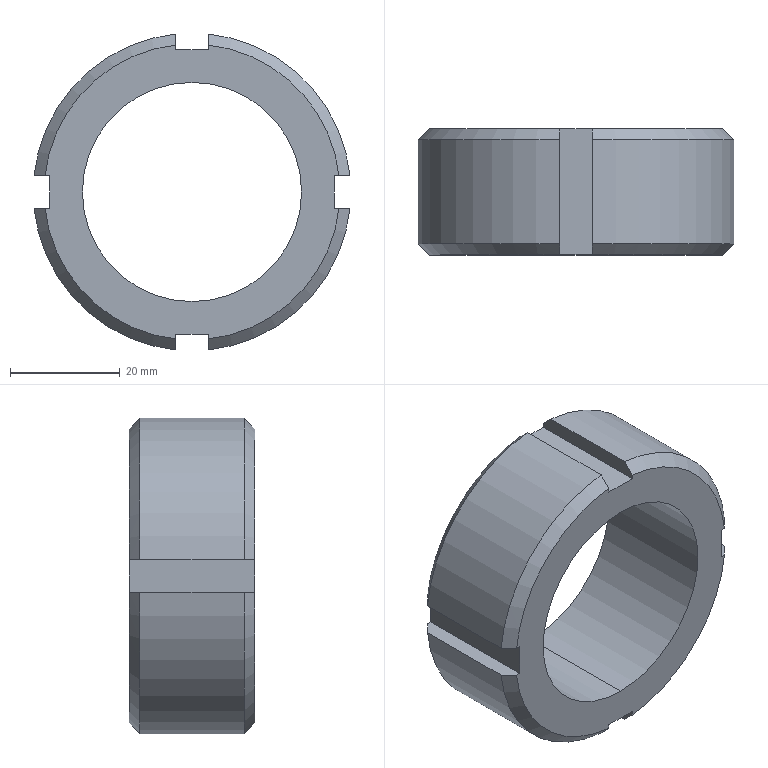Part | SolidWorks | features Chamfer 1, CirPattern 1, Extrusion 1, ICE 1 | 1 solid | 28 faces | box 57.689 x 23 x 57.689 mm | volume 29622 mm3 | plane 14 | cone 8 | cylinder 6 | commonest cylinder face diameters 58 x4 40 x2
STEP:
#1=CARTESIAN_POINT('',(0.,23.,-20.));
#2=VERTEX_POINT('',#1);
#3=CARTESIAN_POINT('',(0.,23.,20.));
#4=VERTEX_POINT('',#3);
#5=CARTESIAN_POINT('',(0.,23.,0.));
#6=DIRECTION('',(0.,1.,0.));
#7=DIRECTION('',(0.,0.,1.));
#8=AXIS2_PLACEMENT_3D('',#5,#6,#7);
#9=CIRCLE('',#8,20.);
#10=EDGE_CURVE('',#2,#4,#9,.T.);
#11=ORIENTED_EDGE('',*,*,#10,.T.);
#12=CARTESIAN_POINT('',(0.,0.,20.));
#13=VERTEX_POINT('',#12);
#14=CARTESIAN_POINT('',(0.,23.,20.));
#15=DIRECTION('',(0.,-1.,0.));
#16=VECTOR('',#15,1000.);
#17=LINE('',#14,#16);
#18=EDGE_CURVE('',#4,#13,#17,.T.);
#19=ORIENTED_EDGE('',*,*,#18,.T.);
#20=CARTESIAN_POINT('',(0.,0.,-20.));
#21=VERTEX_POINT('',#20);
#22=CARTESIAN_POINT('',(0.,0.,0.));
#23=DIRECTION('',(0.,1.,0.));
#24=DIRECTION('',(0.,0.,1.));
#25=AXIS2_PLACEMENT_3D('',#22,#23,#24);
#26=CIRCLE('',#25,20.);
#27=EDGE_CURVE('',#21,#13,#26,.T.);
#28=ORIENTED_EDGE('',*,*,#27,.F.);
#29=CARTESIAN_POINT('',(0.,23.,-20.));
#30=DIRECTION('',(0.,-1.,0.));
#31=VECTOR('',#30,1000.);
#32=LINE('',#29,#31);
#33=EDGE_CURVE('',#2,#21,#32,.T.);
#34=ORIENTED_EDGE('',*,*,#33,.F.);
#35=EDGE_LOOP('',(#11,#19,#28,#34));
#36=FACE_OUTER_BOUND('',#35,.T.);
#37=CARTESIAN_POINT('',(0.,23.,0.));
#38=DIRECTION('',(0.,-1.,0.));
#39=DIRECTION('',(0.,0.,-1.));
#40=AXIS2_PLACEMENT_3D('',#37,#38,#39);
#41=CYLINDRICAL_SURFACE('',#40,20.);
#42=ADVANCED_FACE('',(#36),#41,.F.);
#43=CARTESIAN_POINT('',(28.844,21.,3.));
#44=VERTEX_POINT('',#43);
#45=CARTESIAN_POINT('',(3.,21.,28.844));
#46=VERTEX_POINT('',#45);
#47=CARTESIAN_POINT('',(0.,21.,0.));
#48=DIRECTION('',(0.,-1.,0.));
#49=DIRECTION('',(0.,0.,1.));
#50=AXIS2_PLACEMENT_3D('',#47,#48,#49);
#51=CIRCLE('',#50,29.);
#52=EDGE_CURVE('',#44,#46,#51,.T.);
#53=ORIENTED_EDGE('',*,*,#52,.T.);
#54=CARTESIAN_POINT('',(3.,2.,28.844));
#55=VERTEX_POINT('',#54);
#56=CARTESIAN_POINT('',(3.,23.,28.844));
#57=DIRECTION('',(0.,-1.,0.));
#58=VECTOR('',#57,1000.);
#59=LINE('',#56,#58);
#60=EDGE_CURVE('',#46,#55,#59,.T.);
#61=ORIENTED_EDGE('',*,*,#60,.T.);
#62=CARTESIAN_POINT('',(28.844,2.,3.));
#63=VERTEX_POINT('',#62);
#64=CARTESIAN_POINT('',(0.,2.,0.));
#65=DIRECTION('',(0.,1.,0.));
#66=DIRECTION('',(0.,0.,1.));
#67=AXIS2_PLACEMENT_3D('',#64,#65,#66);
#68=CIRCLE('',#67,29.);
#69=EDGE_CURVE('',#55,#63,#68,.T.);
#70=ORIENTED_EDGE('',*,*,#69,.T.);
#71=CARTESIAN_POINT('',(28.844,23.,3.));
#72=DIRECTION('',(0.,1.,0.));
#73=VECTOR('',#72,1000.);
#74=LINE('',#71,#73);
#75=EDGE_CURVE('',#63,#44,#74,.T.);
#76=ORIENTED_EDGE('',*,*,#75,.T.);
#77=EDGE_LOOP('',(#53,#61,#70,#76));
#78=FACE_OUTER_BOUND('',#77,.T.);
#79=CARTESIAN_POINT('',(0.,23.,0.));
#80=DIRECTION('',(0.,-1.,0.));
#81=DIRECTION('',(0.,0.,-1.));
#82=AXIS2_PLACEMENT_3D('',#79,#80,#81);
#83=CYLINDRICAL_SURFACE('',#82,29.);
#84=ADVANCED_FACE('',(#78),#83,.T.);
#85=CARTESIAN_POINT('',(-28.844,2.,3.));
#86=VERTEX_POINT('',#85);
#87=CARTESIAN_POINT('',(-3.,2.,28.844));
#88=VERTEX_POINT('',#87);
#89=CARTESIAN_POINT('',(0.,2.,0.));
#90=DIRECTION('',(0.,1.,0.));
#91=DIRECTION('',(0.,0.,1.));
#92=AXIS2_PLACEMENT_3D('',#89,#90,#91);
#93=CIRCLE('',#92,29.);
#94=EDGE_CURVE('',#86,#88,#93,.T.);
#95=ORIENTED_EDGE('',*,*,#94,.T.);
#96=CARTESIAN_POINT('',(-3.,21.,28.844));
#97=VERTEX_POINT('',#96);
#98=CARTESIAN_POINT('',(-3.,23.,28.844));
#99=DIRECTION('',(0.,1.,0.));
#100=VECTOR('',#99,1000.);
#101=LINE('',#98,#100);
#102=EDGE_CURVE('',#88,#97,#101,.T.);
#103=ORIENTED_EDGE('',*,*,#102,.T.);
#104=CARTESIAN_POINT('',(-28.844,21.,3.));
#105=VERTEX_POINT('',#104);
#106=CARTESIAN_POINT('',(0.,21.,0.));
#107=DIRECTION('',(0.,-1.,0.));
#108=DIRECTION('',(0.,0.,1.));
#109=AXIS2_PLACEMENT_3D('',#106,#107,#108);
#110=CIRCLE('',#109,29.);
#111=EDGE_CURVE('',#97,#105,#110,.T.);
#112=ORIENTED_EDGE('',*,*,#111,.T.);
#113=CARTESIAN_POINT('',(-28.844,23.,3.));
#114=DIRECTION('',(0.,-1.,0.));
#115=VECTOR('',#114,1000.);
#116=LINE('',#113,#115);
#117=EDGE_CURVE('',#105,#86,#116,.T.);
#118=ORIENTED_EDGE('',*,*,#117,.T.);
#119=EDGE_LOOP('',(#95,#103,#112,#118));
#120=FACE_OUTER_BOUND('',#119,.T.);
#121=CARTESIAN_POINT('',(0.,23.,0.));
#122=DIRECTION('',(0.,-1.,0.));
#123=DIRECTION('',(0.,0.,-1.));
#124=AXIS2_PLACEMENT_3D('',#121,#122,#123);
#125=CYLINDRICAL_SURFACE('',#124,29.);
#126=ADVANCED_FACE('',(#120),#125,.T.);
#127=CARTESIAN_POINT('',(3.,0.,26.833));
#128=VERTEX_POINT('',#127);
#129=CARTESIAN_POINT('',(3.,0.,26.833));
#130=CARTESIAN_POINT('',(3.,0.1315,26.965));
#131=CARTESIAN_POINT('',(3.,0.263,27.097));
#132=CARTESIAN_POINT('',(3.,0.3946,27.23));
#133=CARTESIAN_POINT('',(3.,0.9296,27.768));
#134=CARTESIAN_POINT('',(3.,1.465,28.306));
#135=CARTESIAN_POINT('',(3.,2.,28.844));
#136=B_SPLINE_CURVE_WITH_KNOTS('',3,(#129,#130,#131,#132,#133,#134,#135),.UNSPECIFIED.,.F.,.F.,(4,3,4),(0.006406,0.006966,0.009243),.UNSPECIFIED.);
#137=EDGE_CURVE('',#128,#55,#136,.T.);
#138=ORIENTED_EDGE('',*,*,#137,.F.);
#139=CARTESIAN_POINT('',(26.833,0.,3.));
#140=VERTEX_POINT('',#139);
#141=CARTESIAN_POINT('',(0.,0.,0.));
#142=DIRECTION('',(0.,-1.,0.));
#143=DIRECTION('',(0.,0.,1.));
#144=AXIS2_PLACEMENT_3D('',#141,#142,#143);
#145=CIRCLE('',#144,27.);
#146=EDGE_CURVE('',#140,#128,#145,.T.);
#147=ORIENTED_EDGE('',*,*,#146,.F.);
#148=CARTESIAN_POINT('',(28.844,2.,3.));
#149=CARTESIAN_POINT('',(28.306,1.465,3.));
#150=CARTESIAN_POINT('',(27.768,0.9296,3.));
#151=CARTESIAN_POINT('',(27.23,0.3946,3.));
#152=CARTESIAN_POINT('',(27.097,0.263,3.));
#153=CARTESIAN_POINT('',(26.965,0.1315,3.));
#154=CARTESIAN_POINT('',(26.833,0.,3.));
#155=B_SPLINE_CURVE_WITH_KNOTS('',3,(#148,#149,#150,#151,#152,#153,#154),.UNSPECIFIED.,.F.,.F.,(4,3,4),(0.004689,0.006966,0.007525),.UNSPECIFIED.);
#156=EDGE_CURVE('',#63,#140,#155,.T.);
#157=ORIENTED_EDGE('',*,*,#156,.F.);
#158=ORIENTED_EDGE('',*,*,#69,.F.);
#159=EDGE_LOOP('',(#138,#147,#157,#158));
#160=FACE_OUTER_BOUND('',#159,.T.);
#161=CARTESIAN_POINT('',(0.,2.,0.));
#162=DIRECTION('',(0.,1.,0.));
#163=DIRECTION('',(0.,0.,1.));
#164=AXIS2_PLACEMENT_3D('',#161,#162,#163);
#165=CONICAL_SURFACE('',#164,29.,0.7854);
#166=ADVANCED_FACE('',(#160),#165,.T.);
#167=CARTESIAN_POINT('',(-3.,0.,26.833));
#168=VERTEX_POINT('',#167);
#169=CARTESIAN_POINT('',(-3.,2.,28.844));
#170=CARTESIAN_POINT('',(-3.,1.465,28.306));
#171=CARTESIAN_POINT('',(-3.,0.9296,27.768));
#172=CARTESIAN_POINT('',(-3.,0.3946,27.23));
#173=CARTESIAN_POINT('',(-3.,0.263,27.097));
#174=CARTESIAN_POINT('',(-3.,0.1315,26.965));
#175=CARTESIAN_POINT('',(-3.,0.,26.833));
#176=B_SPLINE_CURVE_WITH_KNOTS('',3,(#169,#170,#171,#172,#173,#174,#175),.UNSPECIFIED.,.F.,.F.,(4,3,4),(0.004689,0.006966,0.007525),.UNSPECIFIED.);
#177=EDGE_CURVE('',#88,#168,#176,.T.);
#178=ORIENTED_EDGE('',*,*,#177,.F.);
#179=ORIENTED_EDGE('',*,*,#94,.F.);
#180=CARTESIAN_POINT('',(-26.833,0.,3.));
#181=VERTEX_POINT('',#180);
#182=CARTESIAN_POINT('',(-26.833,0.,3.));
#183=CARTESIAN_POINT('',(-27.091,0.2565,3.));
#184=CARTESIAN_POINT('',(-27.349,0.513,3.));
#185=CARTESIAN_POINT('',(-27.607,0.7695,3.));
#186=CARTESIAN_POINT('',(-28.02,1.18,3.));
#187=CARTESIAN_POINT('',(-28.432,1.59,3.));
#188=CARTESIAN_POINT('',(-28.844,2.,3.));
#189=B_SPLINE_CURVE_WITH_KNOTS('',3,(#182,#183,#184,#185,#186,#187,#188),.UNSPECIFIED.,.F.,.F.,(4,3,4),(0.005874,0.006966,0.008711),.UNSPECIFIED.);
#190=EDGE_CURVE('',#181,#86,#189,.T.);
#191=ORIENTED_EDGE('',*,*,#190,.F.);
#192=CARTESIAN_POINT('',(0.,0.,0.));
#193=DIRECTION('',(0.,-1.,0.));
#194=DIRECTION('',(0.,0.,1.));
#195=AXIS2_PLACEMENT_3D('',#192,#193,#194);
#196=CIRCLE('',#195,27.);
#197=EDGE_CURVE('',#168,#181,#196,.T.);
#198=ORIENTED_EDGE('',*,*,#197,.F.);
#199=EDGE_LOOP('',(#178,#179,#191,#198));
#200=FACE_OUTER_BOUND('',#199,.T.);
#201=CARTESIAN_POINT('',(0.,2.,0.));
#202=DIRECTION('',(0.,1.,0.));
#203=DIRECTION('',(0.,0.,1.));
#204=AXIS2_PLACEMENT_3D('',#201,#202,#203);
#205=CONICAL_SURFACE('',#204,29.,0.7854);
#206=ADVANCED_FACE('',(#200),#205,.T.);
#207=CARTESIAN_POINT('',(3.,23.,26.833));
#208=VERTEX_POINT('',#207);
#209=CARTESIAN_POINT('',(3.,21.,28.844));
#210=CARTESIAN_POINT('',(3.,21.535,28.306));
#211=CARTESIAN_POINT('',(3.,22.07,27.768));
#212=CARTESIAN_POINT('',(3.,22.605,27.23));
#213=CARTESIAN_POINT('',(3.,22.737,27.097));
#214=CARTESIAN_POINT('',(3.,22.868,26.965));
#215=CARTESIAN_POINT('',(3.,23.,26.833));
#216=B_SPLINE_CURVE_WITH_KNOTS('',3,(#209,#210,#211,#212,#213,#214,#215),.UNSPECIFIED.,.F.,.F.,(4,3,4),(0.004689,0.006966,0.007525),.UNSPECIFIED.);
#217=EDGE_CURVE('',#46,#208,#216,.T.);
#218=ORIENTED_EDGE('',*,*,#217,.F.);
#219=ORIENTED_EDGE('',*,*,#52,.F.);
#220=CARTESIAN_POINT('',(26.833,23.,3.));
#221=VERTEX_POINT('',#220);
#222=CARTESIAN_POINT('',(26.833,23.,3.));
#223=CARTESIAN_POINT('',(26.965,22.868,3.));
#224=CARTESIAN_POINT('',(27.097,22.737,3.));
#225=CARTESIAN_POINT('',(27.23,22.605,3.));
#226=CARTESIAN_POINT('',(27.768,22.07,3.));
#227=CARTESIAN_POINT('',(28.306,21.535,3.));
#228=CARTESIAN_POINT('',(28.844,21.,3.));
#229=B_SPLINE_CURVE_WITH_KNOTS('',3,(#222,#223,#224,#225,#226,#227,#228),.UNSPECIFIED.,.F.,.F.,(4,3,4),(0.006406,0.006966,0.009243),.UNSPECIFIED.);
#230=EDGE_CURVE('',#221,#44,#229,.T.);
#231=ORIENTED_EDGE('',*,*,#230,.F.);
#232=CARTESIAN_POINT('',(0.,23.,0.));
#233=DIRECTION('',(0.,1.,0.));
#234=DIRECTION('',(0.,0.,1.));
#235=AXIS2_PLACEMENT_3D('',#232,#233,#234);
#236=CIRCLE('',#235,27.);
#237=EDGE_CURVE('',#208,#221,#236,.T.);
#238=ORIENTED_EDGE('',*,*,#237,.F.);
#239=EDGE_LOOP('',(#218,#219,#231,#238));
#240=FACE_OUTER_BOUND('',#239,.T.);
#241=CARTESIAN_POINT('',(0.,23.,0.));
#242=DIRECTION('',(0.,-1.,0.));
#243=DIRECTION('',(0.,0.,-1.));
#244=AXIS2_PLACEMENT_3D('',#241,#242,#243);
#245=CONICAL_SURFACE('',#244,27.,0.7854);
#246=ADVANCED_FACE('',(#240),#245,.T.);
#247=CARTESIAN_POINT('',(-3.,23.,26.833));
#248=VERTEX_POINT('',#247);
#249=CARTESIAN_POINT('',(-3.,23.,26.833));
#250=CARTESIAN_POINT('',(-3.,22.868,26.965));
#251=CARTESIAN_POINT('',(-3.,22.737,27.097));
#252=CARTESIAN_POINT('',(-3.,22.605,27.23));
#253=CARTESIAN_POINT('',(-3.,22.07,27.768));
#254=CARTESIAN_POINT('',(-3.,21.535,28.306));
#255=CARTESIAN_POINT('',(-3.,21.,28.844));
#256=B_SPLINE_CURVE_WITH_KNOTS('',3,(#249,#250,#251,#252,#253,#254,#255),.UNSPECIFIED.,.F.,.F.,(4,3,4),(0.006406,0.006966,0.009243),.UNSPECIFIED.);
#257=EDGE_CURVE('',#248,#97,#256,.T.);
#258=ORIENTED_EDGE('',*,*,#257,.F.);
#259=CARTESIAN_POINT('',(-26.833,23.,3.));
#260=VERTEX_POINT('',#259);
#261=CARTESIAN_POINT('',(0.,23.,0.));
#262=DIRECTION('',(0.,1.,0.));
#263=DIRECTION('',(0.,0.,1.));
#264=AXIS2_PLACEMENT_3D('',#261,#262,#263);
#265=CIRCLE('',#264,27.);
#266=EDGE_CURVE('',#260,#248,#265,.T.);
#267=ORIENTED_EDGE('',*,*,#266,.F.);
#268=CARTESIAN_POINT('',(-28.844,21.,3.));
#269=CARTESIAN_POINT('',(-28.724,21.119,3.));
#270=CARTESIAN_POINT('',(-28.604,21.239,3.));
#271=CARTESIAN_POINT('',(-28.484,21.358,3.));
#272=CARTESIAN_POINT('',(-27.934,21.906,3.));
#273=CARTESIAN_POINT('',(-27.383,22.453,3.));
#274=CARTESIAN_POINT('',(-26.833,23.,3.));
#275=B_SPLINE_CURVE_WITH_KNOTS('',3,(#268,#269,#270,#271,#272,#273,#274),.UNSPECIFIED.,.F.,.F.,(4,3,4),(0.006458,0.006966,0.009294),.UNSPECIFIED.);
#276=EDGE_CURVE('',#105,#260,#275,.T.);
#277=ORIENTED_EDGE('',*,*,#276,.F.);
#278=ORIENTED_EDGE('',*,*,#111,.F.);
#279=EDGE_LOOP('',(#258,#267,#277,#278));
#280=FACE_OUTER_BOUND('',#279,.T.);
#281=CARTESIAN_POINT('',(0.,23.,0.));
#282=DIRECTION('',(0.,-1.,0.));
#283=DIRECTION('',(0.,0.,-1.));
#284=AXIS2_PLACEMENT_3D('',#281,#282,#283);
#285=CONICAL_SURFACE('',#284,27.,0.7854);
#286=ADVANCED_FACE('',(#280),#285,.T.);
#287=CARTESIAN_POINT('',(3.,21.,-28.844));
#288=VERTEX_POINT('',#287);
#289=CARTESIAN_POINT('',(28.844,21.,-3.));
#290=VERTEX_POINT('',#289);
#291=CARTESIAN_POINT('',(0.,21.,0.));
#292=DIRECTION('',(0.,-1.,0.));
#293=DIRECTION('',(0.,0.,1.));
#294=AXIS2_PLACEMENT_3D('',#291,#292,#293);
#295=CIRCLE('',#294,29.);
#296=EDGE_CURVE('',#288,#290,#295,.T.);
#297=ORIENTED_EDGE('',*,*,#296,.T.);
#298=CARTESIAN_POINT('',(28.844,2.,-3.));
#299=VERTEX_POINT('',#298);
#300=CARTESIAN_POINT('',(28.844,23.,-3.));
#301=DIRECTION('',(0.,-1.,0.));
#302=VECTOR('',#301,1000.);
#303=LINE('',#300,#302);
#304=EDGE_CURVE('',#290,#299,#303,.T.);
#305=ORIENTED_EDGE('',*,*,#304,.T.);
#306=CARTESIAN_POINT('',(3.,2.,-28.844));
#307=VERTEX_POINT('',#306);
#308=CARTESIAN_POINT('',(0.,2.,0.));
#309=DIRECTION('',(0.,1.,0.));
#310=DIRECTION('',(0.,0.,1.));
#311=AXIS2_PLACEMENT_3D('',#308,#309,#310);
#312=CIRCLE('',#311,29.);
#313=EDGE_CURVE('',#299,#307,#312,.T.);
#314=ORIENTED_EDGE('',*,*,#313,.T.);
#315=CARTESIAN_POINT('',(3.,23.,-28.844));
#316=DIRECTION('',(0.,1.,0.));
#317=VECTOR('',#316,1000.);
#318=LINE('',#315,#317);
#319=EDGE_CURVE('',#307,#288,#318,.T.);
#320=ORIENTED_EDGE('',*,*,#319,.T.);
#321=EDGE_LOOP('',(#297,#305,#314,#320));
#322=FACE_OUTER_BOUND('',#321,.T.);
#323=CARTESIAN_POINT('',(0.,23.,0.));
#324=DIRECTION('',(0.,-1.,0.));
#325=DIRECTION('',(0.,0.,-1.));
#326=AXIS2_PLACEMENT_3D('',#323,#324,#325);
#327=CYLINDRICAL_SURFACE('',#326,29.);
#328=ADVANCED_FACE('',(#322),#327,.T.);
#329=CARTESIAN_POINT('',(26.833,0.,-3.));
#330=VERTEX_POINT('',#329);
#331=CARTESIAN_POINT('',(26.833,0.,-3.));
#332=CARTESIAN_POINT('',(26.965,0.1315,-3.));
#333=CARTESIAN_POINT('',(27.097,0.263,-3.));
#334=CARTESIAN_POINT('',(27.23,0.3946,-3.));
#335=CARTESIAN_POINT('',(27.768,0.9296,-3.));
#336=CARTESIAN_POINT('',(28.306,1.465,-3.));
#337=CARTESIAN_POINT('',(28.844,2.,-3.));
#338=B_SPLINE_CURVE_WITH_KNOTS('',3,(#331,#332,#333,#334,#335,#336,#337),.UNSPECIFIED.,.F.,.F.,(4,3,4),(0.006406,0.006966,0.009243),.UNSPECIFIED.);
#339=EDGE_CURVE('',#330,#299,#338,.T.);
#340=ORIENTED_EDGE('',*,*,#339,.F.);
#341=CARTESIAN_POINT('',(3.,0.,-26.833));
#342=VERTEX_POINT('',#341);
#343=CARTESIAN_POINT('',(0.,0.,0.));
#344=DIRECTION('',(0.,-1.,0.));
#345=DIRECTION('',(0.,0.,1.));
#346=AXIS2_PLACEMENT_3D('',#343,#344,#345);
#347=CIRCLE('',#346,27.);
#348=EDGE_CURVE('',#342,#330,#347,.T.);
#349=ORIENTED_EDGE('',*,*,#348,.F.);
#350=CARTESIAN_POINT('',(3.,2.,-28.844));
#351=CARTESIAN_POINT('',(3.,1.59,-28.432));
#352=CARTESIAN_POINT('',(3.,1.18,-28.02));
#353=CARTESIAN_POINT('',(3.,0.7695,-27.607));
#354=CARTESIAN_POINT('',(3.,0.513,-27.349));
#355=CARTESIAN_POINT('',(3.,0.2565,-27.091));
#356=CARTESIAN_POINT('',(3.,0.,-26.833));
#357=B_SPLINE_CURVE_WITH_KNOTS('',3,(#350,#351,#352,#353,#354,#355,#356),.UNSPECIFIED.,.F.,.F.,(4,3,4),(0.005221,0.006966,0.008057),.UNSPECIFIED.);
#358=EDGE_CURVE('',#307,#342,#357,.T.);
#359=ORIENTED_EDGE('',*,*,#358,.F.);
#360=ORIENTED_EDGE('',*,*,#313,.F.);
#361=EDGE_LOOP('',(#340,#349,#359,#360));
#362=FACE_OUTER_BOUND('',#361,.T.);
#363=CARTESIAN_POINT('',(0.,2.,0.));
#364=DIRECTION('',(0.,1.,0.));
#365=DIRECTION('',(0.,0.,1.));
#366=AXIS2_PLACEMENT_3D('',#363,#364,#365);
#367=CONICAL_SURFACE('',#366,29.,0.7854);
#368=ADVANCED_FACE('',(#362),#367,.T.);
#369=CARTESIAN_POINT('',(26.833,23.,-3.));
#370=VERTEX_POINT('',#369);
#371=CARTESIAN_POINT('',(28.844,21.,-3.));
#372=CARTESIAN_POINT('',(28.306,21.535,-3.));
#373=CARTESIAN_POINT('',(27.768,22.07,-3.));
#374=CARTESIAN_POINT('',(27.23,22.605,-3.));
#375=CARTESIAN_POINT('',(27.097,22.737,-3.));
#376=CARTESIAN_POINT('',(26.965,22.868,-3.));
#377=CARTESIAN_POINT('',(26.833,23.,-3.));
#378=B_SPLINE_CURVE_WITH_KNOTS('',3,(#371,#372,#373,#374,#375,#376,#377),.UNSPECIFIED.,.F.,.F.,(4,3,4),(0.004689,0.006966,0.007525),.UNSPECIFIED.);
#379=EDGE_CURVE('',#290,#370,#378,.T.);
#380=ORIENTED_EDGE('',*,*,#379,.F.);
#381=ORIENTED_EDGE('',*,*,#296,.F.);
#382=CARTESIAN_POINT('',(3.,23.,-26.833));
#383=VERTEX_POINT('',#382);
#384=CARTESIAN_POINT('',(3.,23.,-26.833));
#385=CARTESIAN_POINT('',(3.,22.453,-27.383));
#386=CARTESIAN_POINT('',(3.,21.906,-27.934));
#387=CARTESIAN_POINT('',(3.,21.358,-28.484));
#388=CARTESIAN_POINT('',(3.,21.239,-28.604));
#389=CARTESIAN_POINT('',(3.,21.119,-28.724));
#390=CARTESIAN_POINT('',(3.,21.,-28.844));
#391=B_SPLINE_CURVE_WITH_KNOTS('',3,(#384,#385,#386,#387,#388,#389,#390),.UNSPECIFIED.,.F.,.F.,(4,3,4),(0.004637,0.006966,0.007474),.UNSPECIFIED.);
#392=EDGE_CURVE('',#383,#288,#391,.T.);
#393=ORIENTED_EDGE('',*,*,#392,.F.);
#394=CARTESIAN_POINT('',(0.,23.,0.));
#395=DIRECTION('',(0.,1.,0.));
#396=DIRECTION('',(0.,0.,1.));
#397=AXIS2_PLACEMENT_3D('',#394,#395,#396);
#398=CIRCLE('',#397,27.);
#399=EDGE_CURVE('',#370,#383,#398,.T.);
#400=ORIENTED_EDGE('',*,*,#399,.F.);
#401=EDGE_LOOP('',(#380,#381,#393,#400));
#402=FACE_OUTER_BOUND('',#401,.T.);
#403=CARTESIAN_POINT('',(0.,23.,0.));
#404=DIRECTION('',(0.,-1.,0.));
#405=DIRECTION('',(0.,0.,-1.));
#406=AXIS2_PLACEMENT_3D('',#403,#404,#405);
#407=CONICAL_SURFACE('',#406,27.,0.7854);
#408=ADVANCED_FACE('',(#402),#407,.T.);
#409=CARTESIAN_POINT('',(3.,23.,26.));
#410=VERTEX_POINT('',#409);
#411=CARTESIAN_POINT('',(3.,23.,38.437));
#412=DIRECTION('',(0.,0.,-1.));
#413=VECTOR('',#412,1000.);
#414=LINE('',#411,#413);
#415=EDGE_CURVE('',#208,#410,#414,.T.);
#416=ORIENTED_EDGE('',*,*,#415,.F.);
#417=ORIENTED_EDGE('',*,*,#237,.T.);
#418=CARTESIAN_POINT('',(26.,23.,3.));
#419=VERTEX_POINT('',#418);
#420=CARTESIAN_POINT('',(38.437,23.,3.));
#421=DIRECTION('',(1.,0.,0.));
#422=VECTOR('',#421,1000.);
#423=LINE('',#420,#422);
#424=EDGE_CURVE('',#419,#221,#423,.T.);
#425=ORIENTED_EDGE('',*,*,#424,.F.);
#426=CARTESIAN_POINT('',(26.,23.,-3.));
#427=VERTEX_POINT('',#426);
#428=CARTESIAN_POINT('',(26.,23.,-3.));
#429=DIRECTION('',(0.,0.,1.));
#430=VECTOR('',#429,1000.);
#431=LINE('',#428,#430);
#432=EDGE_CURVE('',#427,#419,#431,.T.);
#433=ORIENTED_EDGE('',*,*,#432,.F.);
#434=CARTESIAN_POINT('',(38.437,23.,-3.));
#435=DIRECTION('',(-1.,0.,0.));
#436=VECTOR('',#435,1000.);
#437=LINE('',#434,#436);
#438=EDGE_CURVE('',#370,#427,#437,.T.);
#439=ORIENTED_EDGE('',*,*,#438,.F.);
#440=ORIENTED_EDGE('',*,*,#399,.T.);
#441=CARTESIAN_POINT('',(3.,23.,-26.));
#442=VERTEX_POINT('',#441);
#443=CARTESIAN_POINT('',(3.,23.,-38.437));
#444=DIRECTION('',(0.,0.,-1.));
#445=VECTOR('',#444,1000.);
#446=LINE('',#443,#445);
#447=EDGE_CURVE('',#442,#383,#446,.T.);
#448=ORIENTED_EDGE('',*,*,#447,.F.);
#449=CARTESIAN_POINT('',(-3.,23.,-26.));
#450=VERTEX_POINT('',#449);
#451=CARTESIAN_POINT('',(-3.,23.,-26.));
#452=DIRECTION('',(1.,0.,0.));
#453=VECTOR('',#452,1000.);
#454=LINE('',#451,#453);
#455=EDGE_CURVE('',#450,#442,#454,.T.);
#456=ORIENTED_EDGE('',*,*,#455,.F.);
#457=CARTESIAN_POINT('',(-3.,23.,-26.833));
#458=VERTEX_POINT('',#457);
#459=CARTESIAN_POINT('',(-3.,23.,-38.437));
#460=DIRECTION('',(0.,0.,1.));
#461=VECTOR('',#460,1000.);
#462=LINE('',#459,#461);
#463=EDGE_CURVE('',#458,#450,#462,.T.);
#464=ORIENTED_EDGE('',*,*,#463,.F.);
#465=CARTESIAN_POINT('',(-26.833,23.,-3.));
#466=VERTEX_POINT('',#465);
#467=CARTESIAN_POINT('',(0.,23.,0.));
#468=DIRECTION('',(0.,1.,0.));
#469=DIRECTION('',(0.,0.,1.));
#470=AXIS2_PLACEMENT_3D('',#467,#468,#469);
#471=CIRCLE('',#470,27.);
#472=EDGE_CURVE('',#458,#466,#471,.T.);
#473=ORIENTED_EDGE('',*,*,#472,.T.);
#474=CARTESIAN_POINT('',(-26.,23.,-3.));
#475=VERTEX_POINT('',#474);
#476=CARTESIAN_POINT('',(-38.437,23.,-3.));
#477=DIRECTION('',(-1.,0.,0.));
#478=VECTOR('',#477,1000.);
#479=LINE('',#476,#478);
#480=EDGE_CURVE('',#475,#466,#479,.T.);
#481=ORIENTED_EDGE('',*,*,#480,.F.);
#482=CARTESIAN_POINT('',(-26.,23.,3.));
#483=VERTEX_POINT('',#482);
#484=CARTESIAN_POINT('',(-26.,23.,3.));
#485=DIRECTION('',(0.,0.,-1.));
#486=VECTOR('',#485,1000.);
#487=LINE('',#484,#486);
#488=EDGE_CURVE('',#483,#475,#487,.T.);
#489=ORIENTED_EDGE('',*,*,#488,.F.);
#490=CARTESIAN_POINT('',(-38.437,23.,3.));
#491=DIRECTION('',(1.,0.,0.));
#492=VECTOR('',#491,1000.);
#493=LINE('',#490,#492);
#494=EDGE_CURVE('',#260,#483,#493,.T.);
#495=ORIENTED_EDGE('',*,*,#494,.F.);
#496=ORIENTED_EDGE('',*,*,#266,.T.);
#497=CARTESIAN_POINT('',(-3.,23.,26.));
#498=VERTEX_POINT('',#497);
#499=CARTESIAN_POINT('',(-3.,23.,38.437));
#500=DIRECTION('',(0.,0.,1.));
#501=VECTOR('',#500,1000.);
#502=LINE('',#499,#501);
#503=EDGE_CURVE('',#498,#248,#502,.T.);
#504=ORIENTED_EDGE('',*,*,#503,.F.);
#505=CARTESIAN_POINT('',(3.,23.,26.));
#506=DIRECTION('',(-1.,0.,0.));
#507=VECTOR('',#506,1000.);
#508=LINE('',#505,#507);
#509=EDGE_CURVE('',#410,#498,#508,.T.);
#510=ORIENTED_EDGE('',*,*,#509,.F.);
#511=EDGE_LOOP('',(#416,#417,#425,#433,#439,#440,#448,#456,#464,#473,#481,#489,#495,#496,#504,#510));
#512=FACE_OUTER_BOUND('',#511,.T.);
#513=ORIENTED_EDGE('',*,*,#10,.F.);
#514=CARTESIAN_POINT('',(0.,23.,0.));
#515=DIRECTION('',(0.,1.,0.));
#516=DIRECTION('',(0.,0.,1.));
#517=AXIS2_PLACEMENT_3D('',#514,#515,#516);
#518=CIRCLE('',#517,20.);
#519=EDGE_CURVE('',#4,#2,#518,.T.);
#520=ORIENTED_EDGE('',*,*,#519,.F.);
#521=EDGE_LOOP('',(#513,#520));
#522=FACE_BOUND('',#521,.T.);
#523=CARTESIAN_POINT('',(0.,23.,0.));
#524=DIRECTION('',(0.,1.,0.));
#525=DIRECTION('',(0.,0.,1.));
#526=AXIS2_PLACEMENT_3D('',#523,#524,#525);
#527=PLANE('',#526);
#528=ADVANCED_FACE('',(#512,#522),#527,.T.);
#529=ORIENTED_EDGE('',*,*,#146,.T.);
#530=CARTESIAN_POINT('',(3.,0.,26.));
#531=VERTEX_POINT('',#530);
#532=CARTESIAN_POINT('',(3.,0.,38.437));
#533=DIRECTION('',(0.,0.,-1.));
#534=VECTOR('',#533,1000.);
#535=LINE('',#532,#534);
#536=EDGE_CURVE('',#128,#531,#535,.T.);
#537=ORIENTED_EDGE('',*,*,#536,.T.);
#538=CARTESIAN_POINT('',(-3.,0.,26.));
#539=VERTEX_POINT('',#538);
#540=CARTESIAN_POINT('',(3.,0.,26.));
#541=DIRECTION('',(-1.,0.,0.));
#542=VECTOR('',#541,1000.);
#543=LINE('',#540,#542);
#544=EDGE_CURVE('',#531,#539,#543,.T.);
#545=ORIENTED_EDGE('',*,*,#544,.T.);
#546=CARTESIAN_POINT('',(-3.,0.,38.437));
#547=DIRECTION('',(0.,0.,1.));
#548=VECTOR('',#547,1000.);
#549=LINE('',#546,#548);
#550=EDGE_CURVE('',#539,#168,#549,.T.);
#551=ORIENTED_EDGE('',*,*,#550,.T.);
#552=ORIENTED_EDGE('',*,*,#197,.T.);
#553=CARTESIAN_POINT('',(-26.,0.,3.));
#554=VERTEX_POINT('',#553);
#555=CARTESIAN_POINT('',(-38.437,0.,3.));
#556=DIRECTION('',(1.,0.,0.));
#557=VECTOR('',#556,1000.);
#558=LINE('',#555,#557);
#559=EDGE_CURVE('',#181,#554,#558,.T.);
#560=ORIENTED_EDGE('',*,*,#559,.T.);
#561=CARTESIAN_POINT('',(-26.,0.,-3.));
#562=VERTEX_POINT('',#561);
#563=CARTESIAN_POINT('',(-26.,0.,3.));
#564=DIRECTION('',(0.,0.,-1.));
#565=VECTOR('',#564,1000.);
#566=LINE('',#563,#565);
#567=EDGE_CURVE('',#554,#562,#566,.T.);
#568=ORIENTED_EDGE('',*,*,#567,.T.);
#569=CARTESIAN_POINT('',(-26.833,0.,-3.));
#570=VERTEX_POINT('',#569);
#571=CARTESIAN_POINT('',(-38.437,0.,-3.));
#572=DIRECTION('',(-1.,0.,0.));
#573=VECTOR('',#572,1000.);
#574=LINE('',#571,#573);
#575=EDGE_CURVE('',#562,#570,#574,.T.);
#576=ORIENTED_EDGE('',*,*,#575,.T.);
#577=CARTESIAN_POINT('',(-3.,0.,-26.833));
#578=VERTEX_POINT('',#577);
#579=CARTESIAN_POINT('',(0.,0.,0.));
#580=DIRECTION('',(0.,-1.,0.));
#581=DIRECTION('',(0.,0.,1.));
#582=AXIS2_PLACEMENT_3D('',#579,#580,#581);
#583=CIRCLE('',#582,27.);
#584=EDGE_CURVE('',#570,#578,#583,.T.);
#585=ORIENTED_EDGE('',*,*,#584,.T.);
#586=CARTESIAN_POINT('',(-3.,0.,-26.));
#587=VERTEX_POINT('',#586);
#588=CARTESIAN_POINT('',(-3.,0.,-38.437));
#589=DIRECTION('',(0.,0.,1.));
#590=VECTOR('',#589,1000.);
#591=LINE('',#588,#590);
#592=EDGE_CURVE('',#578,#587,#591,.T.);
#593=ORIENTED_EDGE('',*,*,#592,.T.);
#594=CARTESIAN_POINT('',(3.,0.,-26.));
#595=VERTEX_POINT('',#594);
#596=CARTESIAN_POINT('',(-3.,0.,-26.));
#597=DIRECTION('',(1.,0.,0.));
#598=VECTOR('',#597,1000.);
#599=LINE('',#596,#598);
#600=EDGE_CURVE('',#587,#595,#599,.T.);
#601=ORIENTED_EDGE('',*,*,#600,.T.);
#602=CARTESIAN_POINT('',(3.,0.,-38.437));
#603=DIRECTION('',(0.,0.,-1.));
#604=VECTOR('',#603,1000.);
#605=LINE('',#602,#604);
#606=EDGE_CURVE('',#595,#342,#605,.T.);
#607=ORIENTED_EDGE('',*,*,#606,.T.);
#608=ORIENTED_EDGE('',*,*,#348,.T.);
#609=CARTESIAN_POINT('',(26.,0.,-3.));
#610=VERTEX_POINT('',#609);
#611=CARTESIAN_POINT('',(38.437,0.,-3.));
#612=DIRECTION('',(-1.,0.,0.));
#613=VECTOR('',#612,1000.);
#614=LINE('',#611,#613);
#615=EDGE_CURVE('',#330,#610,#614,.T.);
#616=ORIENTED_EDGE('',*,*,#615,.T.);
#617=CARTESIAN_POINT('',(26.,0.,3.));
#618=VERTEX_POINT('',#617);
#619=CARTESIAN_POINT('',(26.,0.,-3.));
#620=DIRECTION('',(0.,0.,1.));
#621=VECTOR('',#620,1000.);
#622=LINE('',#619,#621);
#623=EDGE_CURVE('',#610,#618,#622,.T.);
#624=ORIENTED_EDGE('',*,*,#623,.T.);
#625=CARTESIAN_POINT('',(38.437,0.,3.));
#626=DIRECTION('',(1.,0.,0.));
#627=VECTOR('',#626,1000.);
#628=LINE('',#625,#627);
#629=EDGE_CURVE('',#618,#140,#628,.T.);
#630=ORIENTED_EDGE('',*,*,#629,.T.);
#631=EDGE_LOOP('',(#529,#537,#545,#551,#552,#560,#568,#576,#585,#593,#601,#607,#608,#616,#624,#630));
#632=FACE_OUTER_BOUND('',#631,.T.);
#633=ORIENTED_EDGE('',*,*,#27,.T.);
#634=CARTESIAN_POINT('',(0.,0.,0.));
#635=DIRECTION('',(0.,1.,0.));
#636=DIRECTION('',(0.,0.,1.));
#637=AXIS2_PLACEMENT_3D('',#634,#635,#636);
#638=CIRCLE('',#637,20.);
#639=EDGE_CURVE('',#13,#21,#638,.T.);
#640=ORIENTED_EDGE('',*,*,#639,.T.);
#641=EDGE_LOOP('',(#633,#640));
#642=FACE_BOUND('',#641,.T.);
#643=CARTESIAN_POINT('',(0.,0.,0.));
#644=DIRECTION('',(0.,1.,0.));
#645=DIRECTION('',(0.,0.,1.));
#646=AXIS2_PLACEMENT_3D('',#643,#644,#645);
#647=PLANE('',#646);
#648=ADVANCED_FACE('',(#632,#642),#647,.F.);
#649=CARTESIAN_POINT('',(-3.,2.,-28.844));
#650=VERTEX_POINT('',#649);
#651=CARTESIAN_POINT('',(-28.844,2.,-3.));
#652=VERTEX_POINT('',#651);
#653=CARTESIAN_POINT('',(0.,2.,0.));
#654=DIRECTION('',(0.,1.,0.));
#655=DIRECTION('',(0.,0.,1.));
#656=AXIS2_PLACEMENT_3D('',#653,#654,#655);
#657=CIRCLE('',#656,29.);
#658=EDGE_CURVE('',#650,#652,#657,.T.);
#659=ORIENTED_EDGE('',*,*,#658,.T.);
#660=CARTESIAN_POINT('',(-28.844,21.,-3.));
#661=VERTEX_POINT('',#660);
#662=CARTESIAN_POINT('',(-28.844,23.,-3.));
#663=DIRECTION('',(0.,1.,0.));
#664=VECTOR('',#663,1000.);
#665=LINE('',#662,#664);
#666=EDGE_CURVE('',#652,#661,#665,.T.);
#667=ORIENTED_EDGE('',*,*,#666,.T.);
#668=CARTESIAN_POINT('',(-3.,21.,-28.844));
#669=VERTEX_POINT('',#668);
#670=CARTESIAN_POINT('',(0.,21.,0.));
#671=DIRECTION('',(0.,-1.,0.));
#672=DIRECTION('',(0.,0.,1.));
#673=AXIS2_PLACEMENT_3D('',#670,#671,#672);
#674=CIRCLE('',#673,29.);
#675=EDGE_CURVE('',#661,#669,#674,.T.);
#676=ORIENTED_EDGE('',*,*,#675,.T.);
#677=CARTESIAN_POINT('',(-3.,23.,-28.844));
#678=DIRECTION('',(0.,-1.,0.));
#679=VECTOR('',#678,1000.);
#680=LINE('',#677,#679);
#681=EDGE_CURVE('',#669,#650,#680,.T.);
#682=ORIENTED_EDGE('',*,*,#681,.T.);
#683=EDGE_LOOP('',(#659,#667,#676,#682));
#684=FACE_OUTER_BOUND('',#683,.T.);
#685=CARTESIAN_POINT('',(0.,23.,0.));
#686=DIRECTION('',(0.,-1.,0.));
#687=DIRECTION('',(0.,0.,-1.));
#688=AXIS2_PLACEMENT_3D('',#685,#686,#687);
#689=CYLINDRICAL_SURFACE('',#688,29.);
#690=ADVANCED_FACE('',(#684),#689,.T.);
#691=ORIENTED_EDGE('',*,*,#18,.F.);
#692=ORIENTED_EDGE('',*,*,#519,.T.);
#693=ORIENTED_EDGE('',*,*,#33,.T.);
#694=ORIENTED_EDGE('',*,*,#639,.F.);
#695=EDGE_LOOP('',(#691,#692,#693,#694));
#696=FACE_OUTER_BOUND('',#695,.T.);
#697=CARTESIAN_POINT('',(0.,23.,0.));
#698=DIRECTION('',(0.,-1.,0.));
#699=DIRECTION('',(0.,0.,-1.));
#700=AXIS2_PLACEMENT_3D('',#697,#698,#699);
#701=CYLINDRICAL_SURFACE('',#700,20.);
#702=ADVANCED_FACE('',(#696),#701,.F.);
#703=CARTESIAN_POINT('',(-28.844,2.,-3.));
#704=CARTESIAN_POINT('',(-28.432,1.59,-3.));
#705=CARTESIAN_POINT('',(-28.02,1.18,-3.));
#706=CARTESIAN_POINT('',(-27.607,0.7695,-3.));
#707=CARTESIAN_POINT('',(-27.349,0.513,-3.));
#708=CARTESIAN_POINT('',(-27.091,0.2565,-3.));
#709=CARTESIAN_POINT('',(-26.833,0.,-3.));
#710=B_SPLINE_CURVE_WITH_KNOTS('',3,(#703,#704,#705,#706,#707,#708,#709),.UNSPECIFIED.,.F.,.F.,(4,3,4),(0.005221,0.006966,0.008057),.UNSPECIFIED.);
#711=EDGE_CURVE('',#652,#570,#710,.T.);
#712=ORIENTED_EDGE('',*,*,#711,.F.);
#713=ORIENTED_EDGE('',*,*,#658,.F.);
#714=CARTESIAN_POINT('',(-3.,0.,-26.833));
#715=CARTESIAN_POINT('',(-3.,0.2565,-27.091));
#716=CARTESIAN_POINT('',(-3.,0.513,-27.349));
#717=CARTESIAN_POINT('',(-3.,0.7695,-27.607));
#718=CARTESIAN_POINT('',(-3.,1.18,-28.02));
#719=CARTESIAN_POINT('',(-3.,1.59,-28.432));
#720=CARTESIAN_POINT('',(-3.,2.,-28.844));
#721=B_SPLINE_CURVE_WITH_KNOTS('',3,(#714,#715,#716,#717,#718,#719,#720),.UNSPECIFIED.,.F.,.F.,(4,3,4),(0.005874,0.006966,0.008711),.UNSPECIFIED.);
#722=EDGE_CURVE('',#578,#650,#721,.T.);
#723=ORIENTED_EDGE('',*,*,#722,.F.);
#724=ORIENTED_EDGE('',*,*,#584,.F.);
#725=EDGE_LOOP('',(#712,#713,#723,#724));
#726=FACE_OUTER_BOUND('',#725,.T.);
#727=CARTESIAN_POINT('',(0.,2.,0.));
#728=DIRECTION('',(0.,1.,0.));
#729=DIRECTION('',(0.,0.,1.));
#730=AXIS2_PLACEMENT_3D('',#727,#728,#729);
#731=CONICAL_SURFACE('',#730,29.,0.7854);
#732=ADVANCED_FACE('',(#726),#731,.T.);
#733=CARTESIAN_POINT('',(-26.833,23.,-3.));
#734=CARTESIAN_POINT('',(-27.383,22.453,-3.));
#735=CARTESIAN_POINT('',(-27.934,21.906,-3.));
#736=CARTESIAN_POINT('',(-28.484,21.358,-3.));
#737=CARTESIAN_POINT('',(-28.604,21.239,-3.));
#738=CARTESIAN_POINT('',(-28.724,21.119,-3.));
#739=CARTESIAN_POINT('',(-28.844,21.,-3.));
#740=B_SPLINE_CURVE_WITH_KNOTS('',3,(#733,#734,#735,#736,#737,#738,#739),.UNSPECIFIED.,.F.,.F.,(4,3,4),(0.004637,0.006966,0.007474),.UNSPECIFIED.);
#741=EDGE_CURVE('',#466,#661,#740,.T.);
#742=ORIENTED_EDGE('',*,*,#741,.F.);
#743=ORIENTED_EDGE('',*,*,#472,.F.);
#744=CARTESIAN_POINT('',(-3.,21.,-28.844));
#745=CARTESIAN_POINT('',(-3.,21.119,-28.724));
#746=CARTESIAN_POINT('',(-3.,21.239,-28.604));
#747=CARTESIAN_POINT('',(-3.,21.358,-28.484));
#748=CARTESIAN_POINT('',(-3.,21.906,-27.934));
#749=CARTESIAN_POINT('',(-3.,22.453,-27.383));
#750=CARTESIAN_POINT('',(-3.,23.,-26.833));
#751=B_SPLINE_CURVE_WITH_KNOTS('',3,(#744,#745,#746,#747,#748,#749,#750),.UNSPECIFIED.,.F.,.F.,(4,3,4),(0.006458,0.006966,0.009294),.UNSPECIFIED.);
#752=EDGE_CURVE('',#669,#458,#751,.T.);
#753=ORIENTED_EDGE('',*,*,#752,.F.);
#754=ORIENTED_EDGE('',*,*,#675,.F.);
#755=EDGE_LOOP('',(#742,#743,#753,#754));
#756=FACE_OUTER_BOUND('',#755,.T.);
#757=CARTESIAN_POINT('',(0.,23.,0.));
#758=DIRECTION('',(0.,-1.,0.));
#759=DIRECTION('',(0.,0.,-1.));
#760=AXIS2_PLACEMENT_3D('',#757,#758,#759);
#761=CONICAL_SURFACE('',#760,27.,0.7854);
#762=ADVANCED_FACE('',(#756),#761,.T.);
#763=ORIENTED_EDGE('',*,*,#722,.T.);
#764=ORIENTED_EDGE('',*,*,#681,.F.);
#765=ORIENTED_EDGE('',*,*,#752,.T.);
#766=ORIENTED_EDGE('',*,*,#463,.T.);
#767=CARTESIAN_POINT('',(-3.,0.,-26.));
#768=DIRECTION('',(0.,1.,0.));
#769=VECTOR('',#768,1000.);
#770=LINE('',#767,#769);
#771=EDGE_CURVE('',#587,#450,#770,.T.);
#772=ORIENTED_EDGE('',*,*,#771,.F.);
#773=ORIENTED_EDGE('',*,*,#592,.F.);
#774=EDGE_LOOP('',(#763,#764,#765,#766,#772,#773));
#775=FACE_OUTER_BOUND('',#774,.T.);
#776=CARTESIAN_POINT('',(-3.,0.,-38.437));
#777=DIRECTION('',(-1.,0.,0.));
#778=DIRECTION('',(0.,0.,1.));
#779=AXIS2_PLACEMENT_3D('',#776,#777,#778);
#780=PLANE('',#779);
#781=ADVANCED_FACE('',(#775),#780,.F.);
#782=ORIENTED_EDGE('',*,*,#358,.T.);
#783=ORIENTED_EDGE('',*,*,#606,.F.);
#784=CARTESIAN_POINT('',(3.,0.,-26.));
#785=DIRECTION('',(0.,1.,0.));
#786=VECTOR('',#785,1000.);
#787=LINE('',#784,#786);
#788=EDGE_CURVE('',#595,#442,#787,.T.);
#789=ORIENTED_EDGE('',*,*,#788,.T.);
#790=ORIENTED_EDGE('',*,*,#447,.T.);
#791=ORIENTED_EDGE('',*,*,#392,.T.);
#792=ORIENTED_EDGE('',*,*,#319,.F.);
#793=EDGE_LOOP('',(#782,#783,#789,#790,#791,#792));
#794=FACE_OUTER_BOUND('',#793,.T.);
#795=CARTESIAN_POINT('',(3.,0.,-38.437));
#796=DIRECTION('',(1.,0.,0.));
#797=DIRECTION('',(0.,0.,-1.));
#798=AXIS2_PLACEMENT_3D('',#795,#796,#797);
#799=PLANE('',#798);
#800=ADVANCED_FACE('',(#794),#799,.F.);
#801=ORIENTED_EDGE('',*,*,#455,.T.);
#802=ORIENTED_EDGE('',*,*,#788,.F.);
#803=ORIENTED_EDGE('',*,*,#600,.F.);
#804=ORIENTED_EDGE('',*,*,#771,.T.);
#805=EDGE_LOOP('',(#801,#802,#803,#804));
#806=FACE_OUTER_BOUND('',#805,.T.);
#807=CARTESIAN_POINT('',(-3.,0.,-26.));
#808=DIRECTION('',(0.,0.,1.));
#809=DIRECTION('',(1.,0.,0.));
#810=AXIS2_PLACEMENT_3D('',#807,#808,#809);
#811=PLANE('',#810);
#812=ADVANCED_FACE('',(#806),#811,.F.);
#813=ORIENTED_EDGE('',*,*,#339,.T.);
#814=ORIENTED_EDGE('',*,*,#304,.F.);
#815=ORIENTED_EDGE('',*,*,#379,.T.);
#816=ORIENTED_EDGE('',*,*,#438,.T.);
#817=CARTESIAN_POINT('',(26.,0.,-3.));
#818=DIRECTION('',(0.,1.,0.));
#819=VECTOR('',#818,1000.);
#820=LINE('',#817,#819);
#821=EDGE_CURVE('',#610,#427,#820,.T.);
#822=ORIENTED_EDGE('',*,*,#821,.F.);
#823=ORIENTED_EDGE('',*,*,#615,.F.);
#824=EDGE_LOOP('',(#813,#814,#815,#816,#822,#823));
#825=FACE_OUTER_BOUND('',#824,.T.);
#826=CARTESIAN_POINT('',(38.437,0.,-3.));
#827=DIRECTION('',(0.,0.,-1.));
#828=DIRECTION('',(-1.,0.,0.));
#829=AXIS2_PLACEMENT_3D('',#826,#827,#828);
#830=PLANE('',#829);
#831=ADVANCED_FACE('',(#825),#830,.F.);
#832=ORIENTED_EDGE('',*,*,#156,.T.);
#833=ORIENTED_EDGE('',*,*,#629,.F.);
#834=CARTESIAN_POINT('',(26.,0.,3.));
#835=DIRECTION('',(0.,1.,0.));
#836=VECTOR('',#835,1000.);
#837=LINE('',#834,#836);
#838=EDGE_CURVE('',#618,#419,#837,.T.);
#839=ORIENTED_EDGE('',*,*,#838,.T.);
#840=ORIENTED_EDGE('',*,*,#424,.T.);
#841=ORIENTED_EDGE('',*,*,#230,.T.);
#842=ORIENTED_EDGE('',*,*,#75,.F.);
#843=EDGE_LOOP('',(#832,#833,#839,#840,#841,#842));
#844=FACE_OUTER_BOUND('',#843,.T.);
#845=CARTESIAN_POINT('',(38.437,0.,3.));
#846=DIRECTION('',(0.,0.,1.));
#847=DIRECTION('',(1.,0.,0.));
#848=AXIS2_PLACEMENT_3D('',#845,#846,#847);
#849=PLANE('',#848);
#850=ADVANCED_FACE('',(#844),#849,.F.);
#851=ORIENTED_EDGE('',*,*,#432,.T.);
#852=ORIENTED_EDGE('',*,*,#838,.F.);
#853=ORIENTED_EDGE('',*,*,#623,.F.);
#854=ORIENTED_EDGE('',*,*,#821,.T.);
#855=EDGE_LOOP('',(#851,#852,#853,#854));
#856=FACE_OUTER_BOUND('',#855,.T.);
#857=CARTESIAN_POINT('',(26.,0.,-3.));
#858=DIRECTION('',(-1.,0.,0.));
#859=DIRECTION('',(0.,0.,1.));
#860=AXIS2_PLACEMENT_3D('',#857,#858,#859);
#861=PLANE('',#860);
#862=ADVANCED_FACE('',(#856),#861,.F.);
#863=ORIENTED_EDGE('',*,*,#190,.T.);
#864=ORIENTED_EDGE('',*,*,#117,.F.);
#865=ORIENTED_EDGE('',*,*,#276,.T.);
#866=ORIENTED_EDGE('',*,*,#494,.T.);
#867=CARTESIAN_POINT('',(-26.,0.,3.));
#868=DIRECTION('',(0.,1.,0.));
#869=VECTOR('',#868,1000.);
#870=LINE('',#867,#869);
#871=EDGE_CURVE('',#554,#483,#870,.T.);
#872=ORIENTED_EDGE('',*,*,#871,.F.);
#873=ORIENTED_EDGE('',*,*,#559,.F.);
#874=EDGE_LOOP('',(#863,#864,#865,#866,#872,#873));
#875=FACE_OUTER_BOUND('',#874,.T.);
#876=CARTESIAN_POINT('',(-38.437,0.,3.));
#877=DIRECTION('',(0.,0.,1.));
#878=DIRECTION('',(1.,0.,0.));
#879=AXIS2_PLACEMENT_3D('',#876,#877,#878);
#880=PLANE('',#879);
#881=ADVANCED_FACE('',(#875),#880,.F.);
#882=ORIENTED_EDGE('',*,*,#711,.T.);
#883=ORIENTED_EDGE('',*,*,#575,.F.);
#884=CARTESIAN_POINT('',(-26.,0.,-3.));
#885=DIRECTION('',(0.,1.,0.));
#886=VECTOR('',#885,1000.);
#887=LINE('',#884,#886);
#888=EDGE_CURVE('',#562,#475,#887,.T.);
#889=ORIENTED_EDGE('',*,*,#888,.T.);
#890=ORIENTED_EDGE('',*,*,#480,.T.);
#891=ORIENTED_EDGE('',*,*,#741,.T.);
#892=ORIENTED_EDGE('',*,*,#666,.F.);
#893=EDGE_LOOP('',(#882,#883,#889,#890,#891,#892));
#894=FACE_OUTER_BOUND('',#893,.T.);
#895=CARTESIAN_POINT('',(-38.437,0.,-3.));
#896=DIRECTION('',(0.,0.,-1.));
#897=DIRECTION('',(-1.,0.,0.));
#898=AXIS2_PLACEMENT_3D('',#895,#896,#897);
#899=PLANE('',#898);
#900=ADVANCED_FACE('',(#894),#899,.F.);
#901=ORIENTED_EDGE('',*,*,#488,.T.);
#902=ORIENTED_EDGE('',*,*,#888,.F.);
#903=ORIENTED_EDGE('',*,*,#567,.F.);
#904=ORIENTED_EDGE('',*,*,#871,.T.);
#905=EDGE_LOOP('',(#901,#902,#903,#904));
#906=FACE_OUTER_BOUND('',#905,.T.);
#907=CARTESIAN_POINT('',(-26.,0.,3.));
#908=DIRECTION('',(1.,0.,0.));
#909=DIRECTION('',(0.,0.,-1.));
#910=AXIS2_PLACEMENT_3D('',#907,#908,#909);
#911=PLANE('',#910);
#912=ADVANCED_FACE('',(#906),#911,.F.);
#913=ORIENTED_EDGE('',*,*,#137,.T.);
#914=ORIENTED_EDGE('',*,*,#60,.F.);
#915=ORIENTED_EDGE('',*,*,#217,.T.);
#916=ORIENTED_EDGE('',*,*,#415,.T.);
#917=CARTESIAN_POINT('',(3.,0.,26.));
#918=DIRECTION('',(0.,1.,0.));
#919=VECTOR('',#918,1000.);
#920=LINE('',#917,#919);
#921=EDGE_CURVE('',#531,#410,#920,.T.);
#922=ORIENTED_EDGE('',*,*,#921,.F.);
#923=ORIENTED_EDGE('',*,*,#536,.F.);
#924=EDGE_LOOP('',(#913,#914,#915,#916,#922,#923));
#925=FACE_OUTER_BOUND('',#924,.T.);
#926=CARTESIAN_POINT('',(3.,0.,38.437));
#927=DIRECTION('',(1.,0.,0.));
#928=DIRECTION('',(0.,0.,-1.));
#929=AXIS2_PLACEMENT_3D('',#926,#927,#928);
#930=PLANE('',#929);
#931=ADVANCED_FACE('',(#925),#930,.F.);
#932=ORIENTED_EDGE('',*,*,#177,.T.);
#933=ORIENTED_EDGE('',*,*,#550,.F.);
#934=CARTESIAN_POINT('',(-3.,0.,26.));
#935=DIRECTION('',(0.,1.,0.));
#936=VECTOR('',#935,1000.);
#937=LINE('',#934,#936);
#938=EDGE_CURVE('',#539,#498,#937,.T.);
#939=ORIENTED_EDGE('',*,*,#938,.T.);
#940=ORIENTED_EDGE('',*,*,#503,.T.);
#941=ORIENTED_EDGE('',*,*,#257,.T.);
#942=ORIENTED_EDGE('',*,*,#102,.F.);
#943=EDGE_LOOP('',(#932,#933,#939,#940,#941,#942));
#944=FACE_OUTER_BOUND('',#943,.T.);
#945=CARTESIAN_POINT('',(-3.,0.,38.437));
#946=DIRECTION('',(-1.,0.,0.));
#947=DIRECTION('',(0.,0.,1.));
#948=AXIS2_PLACEMENT_3D('',#945,#946,#947);
#949=PLANE('',#948);
#950=ADVANCED_FACE('',(#944),#949,.F.);
#951=ORIENTED_EDGE('',*,*,#509,.T.);
#952=ORIENTED_EDGE('',*,*,#938,.F.);
#953=ORIENTED_EDGE('',*,*,#544,.F.);
#954=ORIENTED_EDGE('',*,*,#921,.T.);
#955=EDGE_LOOP('',(#951,#952,#953,#954));
#956=FACE_OUTER_BOUND('',#955,.T.);
#957=CARTESIAN_POINT('',(3.,0.,26.));
#958=DIRECTION('',(0.,0.,-1.));
#959=DIRECTION('',(-1.,0.,0.));
#960=AXIS2_PLACEMENT_3D('',#957,#958,#959);
#961=PLANE('',#960);
#962=ADVANCED_FACE('',(#956),#961,.F.);
#963=CLOSED_SHELL('',(#42,#84,#126,#166,#206,#246,#286,#328,#368,#408,#528,#648,#690,#702,#732,#762,#781,#800,#812,#831,#850,#862,#881,#900,#912,#931,#950,#962));
#964=MANIFOLD_SOLID_BREP('',#963);
#965=CARTESIAN_POINT('',(0.,0.,0.));
#966=DIRECTION('',(0.,0.,1.));
#967=DIRECTION('',(1.,0.,0.));
#968=AXIS2_PLACEMENT_3D('',#965,#966,#967);
#969=(LENGTH_UNIT()NAMED_UNIT(*)SI_UNIT(.MILLI.,.METRE.));
#970=UNCERTAINTY_MEASURE_WITH_UNIT(LENGTH_MEASURE(0.00001),#969,'','');
#971=(NAMED_UNIT(*)PLANE_ANGLE_UNIT()SI_UNIT($,.RADIAN.));
#972=(NAMED_UNIT(*)SI_UNIT($,.STERADIAN.)SOLID_ANGLE_UNIT());
#973=(GEOMETRIC_REPRESENTATION_CONTEXT(3)GLOBAL_UNCERTAINTY_ASSIGNED_CONTEXT((#970))GLOBAL_UNIT_ASSIGNED_CONTEXT((#969,#971,#972))REPRESENTATION_CONTEXT('',''));
#974=ADVANCED_BREP_SHAPE_REPRESENTATION('',(#964,#968),#973);